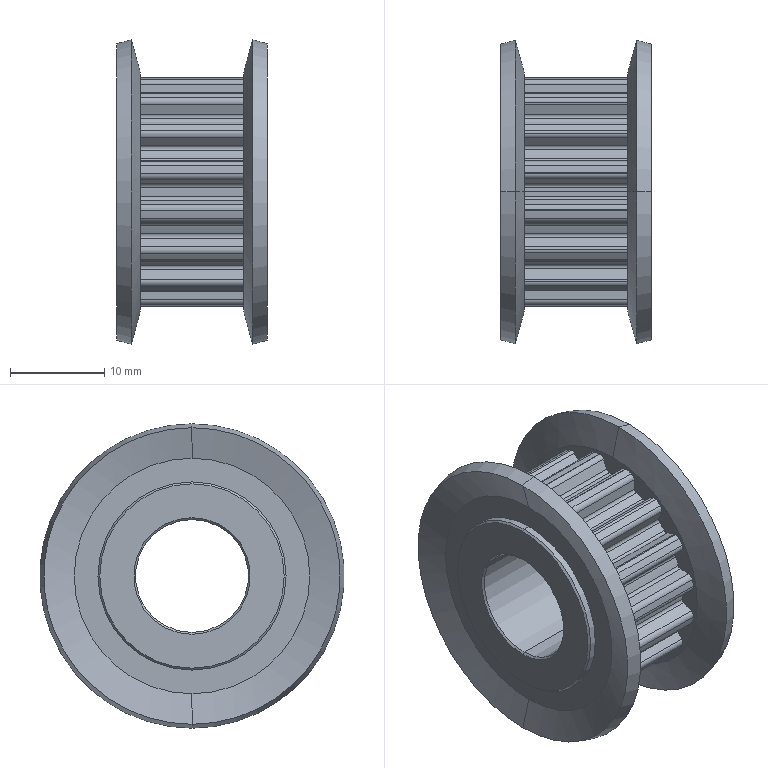Part | SolidWorks | features ICE 1, Revolution 1 | 1 solid | 169 faces | box 16 x 32.358 x 32.358 mm | volume 5839 mm3 | cylinder 115 | plane 38 | cone 16 | commonest cylinder face diameters 0.8 x38 1.2 x38 21 x17 24.6 x16 20 x4 12 x2